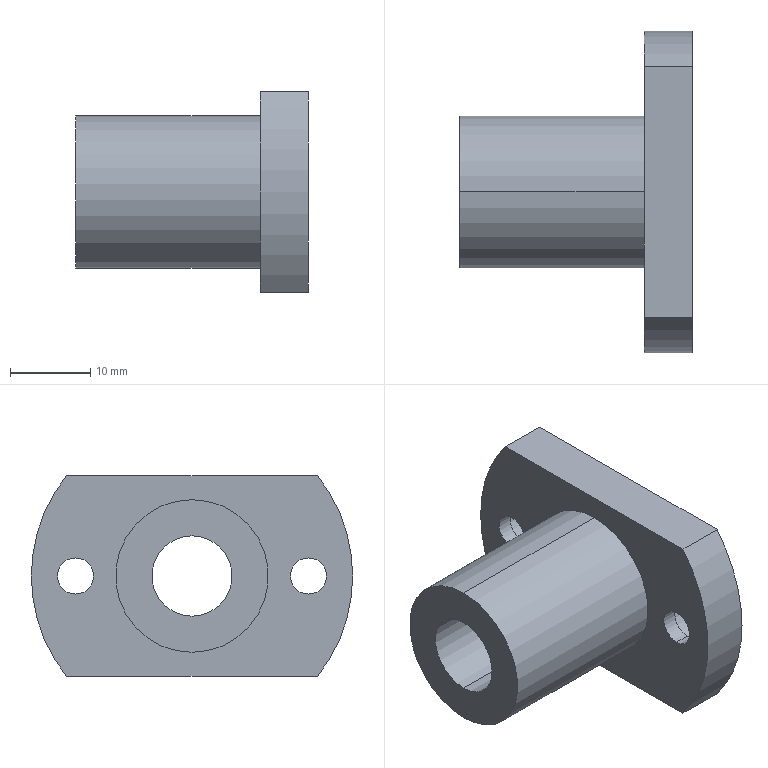Part | STEP file | Linear bearing LHFC 10 | 1 solid | 21 faces | box 29 x 40 x 25 mm | volume 9403 mm3 | cylinder 14 | plane 7 | commonest cylinder face diameters 4.5 x4 7.5 x4 10 x2 19 x2 40 x2
STEP:
#1=CARTESIAN_POINT('',(0.,0.,0.));
#2=DIRECTION('',(0.,0.,1.));
#3=DIRECTION('',(1.,0.,0.));
#4=AXIS2_PLACEMENT_3D('',#1,#2,#3);
#5=CARTESIAN_POINT('',(-23.,0.,9.5));
#6=VERTEX_POINT('',#5);
#7=CARTESIAN_POINT('',(-23.,0.,-9.5));
#8=VERTEX_POINT('',#7);
#9=CARTESIAN_POINT('',(-23.,0.,0.));
#10=DIRECTION('',(-1.,0.,0.));
#11=DIRECTION('',(0.,0.,-1.));
#12=AXIS2_PLACEMENT_3D('',#9,#10,#11);
#13=CIRCLE('',#12,9.5);
#14=CARTESIAN_POINT('',(-23.,0.,0.));
#15=DIRECTION('',(1.,0.,0.));
#16=DIRECTION('',(0.,0.,-1.));
#17=AXIS2_PLACEMENT_3D('',#14,#15,#16);
#18=CYLINDRICAL_SURFACE('',#17,9.5);
#19=CARTESIAN_POINT('',(6.283,0.));
#20=DIRECTION('',(-1.,0.));
#21=VECTOR('',#20,1.);
#22=LINE('',#19,#21);
#23=(GEOMETRIC_REPRESENTATION_CONTEXT(2)PARAMETRIC_REPRESENTATION_CONTEXT()REPRESENTATION_CONTEXT('',''));
#24=DEFINITIONAL_REPRESENTATION('',(#22),#23);
#25=PCURVE('',#18,#24);
#26=CARTESIAN_POINT('',(-23.,-9.614,-9.614));
#27=DIRECTION('',(-1.,0.,0.));
#28=DIRECTION('',(0.,0.,1.));
#29=AXIS2_PLACEMENT_3D('',#26,#27,#28);
#30=PLANE('',#29);
#31=CARTESIAN_POINT('',(9.614,9.614));
#32=DIRECTION('',(-1.,0.));
#33=AXIS2_PLACEMENT_2D('',#31,#32);
#34=CIRCLE('',#33,9.5);
#35=(GEOMETRIC_REPRESENTATION_CONTEXT(2)PARAMETRIC_REPRESENTATION_CONTEXT()REPRESENTATION_CONTEXT('',''));
#36=DEFINITIONAL_REPRESENTATION('',(#34),#35);
#37=PCURVE('',#30,#36);
#38=SURFACE_CURVE('',#13,(#25,#37),.PCURVE_S1.);
#39=EDGE_CURVE('',#6,#8,#38,.T.);
#40=ORIENTED_EDGE('',*,*,#39,.F.);
#41=CARTESIAN_POINT('',(0.,0.,9.5));
#42=VERTEX_POINT('',#41);
#43=CARTESIAN_POINT('',(-23.,0.,9.5));
#44=DIRECTION('',(1.,0.,0.));
#45=VECTOR('',#44,1.);
#46=LINE('',#43,#45);
#47=CARTESIAN_POINT('',(3.142,0.));
#48=DIRECTION('',(0.,1.));
#49=VECTOR('',#48,1.);
#50=LINE('',#47,#49);
#51=(GEOMETRIC_REPRESENTATION_CONTEXT(2)PARAMETRIC_REPRESENTATION_CONTEXT()REPRESENTATION_CONTEXT('',''));
#52=DEFINITIONAL_REPRESENTATION('',(#50),#51);
#53=PCURVE('',#18,#52);
#54=CARTESIAN_POINT('',(-23.,0.,0.));
#55=DIRECTION('',(1.,0.,0.));
#56=DIRECTION('',(0.,0.,-1.));
#57=AXIS2_PLACEMENT_3D('',#54,#55,#56);
#58=CYLINDRICAL_SURFACE('',#57,9.5);
#59=CARTESIAN_POINT('',(3.142,0.));
#60=DIRECTION('',(0.,1.));
#61=VECTOR('',#60,1.);
#62=LINE('',#59,#61);
#63=(GEOMETRIC_REPRESENTATION_CONTEXT(2)PARAMETRIC_REPRESENTATION_CONTEXT()REPRESENTATION_CONTEXT('',''));
#64=DEFINITIONAL_REPRESENTATION('',(#62),#63);
#65=PCURVE('',#58,#64);
#66=SURFACE_CURVE('',#46,(#53,#65),.PCURVE_S1.);
#67=EDGE_CURVE('',#6,#42,#66,.T.);
#68=ORIENTED_EDGE('',*,*,#67,.T.);
#69=CARTESIAN_POINT('',(0.,0.,-9.5));
#70=VERTEX_POINT('',#69);
#71=CARTESIAN_POINT('',(0.,0.,0.));
#72=DIRECTION('',(1.,0.,0.));
#73=DIRECTION('',(0.,0.,-1.));
#74=AXIS2_PLACEMENT_3D('',#71,#72,#73);
#75=CIRCLE('',#74,9.5);
#76=CARTESIAN_POINT('',(0.,23.));
#77=DIRECTION('',(1.,0.));
#78=VECTOR('',#77,1.);
#79=LINE('',#76,#78);
#80=(GEOMETRIC_REPRESENTATION_CONTEXT(2)PARAMETRIC_REPRESENTATION_CONTEXT()REPRESENTATION_CONTEXT('',''));
#81=DEFINITIONAL_REPRESENTATION('',(#79),#80);
#82=PCURVE('',#18,#81);
#83=CARTESIAN_POINT('',(0.,-20.24,12.5));
#84=DIRECTION('',(1.,0.,0.));
#85=DIRECTION('',(0.,0.,-1.));
#86=AXIS2_PLACEMENT_3D('',#83,#84,#85);
#87=PLANE('',#86);
#88=CARTESIAN_POINT('',(12.5,20.24));
#89=DIRECTION('',(1.,0.));
#90=AXIS2_PLACEMENT_2D('',#88,#89);
#91=CIRCLE('',#90,9.5);
#92=(GEOMETRIC_REPRESENTATION_CONTEXT(2)PARAMETRIC_REPRESENTATION_CONTEXT()REPRESENTATION_CONTEXT('',''));
#93=DEFINITIONAL_REPRESENTATION('',(#91),#92);
#94=PCURVE('',#87,#93);
#95=SURFACE_CURVE('',#75,(#82,#94),.PCURVE_S1.);
#96=EDGE_CURVE('',#70,#42,#95,.T.);
#97=ORIENTED_EDGE('',*,*,#96,.F.);
#98=CARTESIAN_POINT('',(-23.,0.,-9.5));
#99=DIRECTION('',(1.,0.,0.));
#100=VECTOR('',#99,1.);
#101=LINE('',#98,#100);
#102=CARTESIAN_POINT('',(0.,0.));
#103=DIRECTION('',(0.,1.));
#104=VECTOR('',#103,1.);
#105=LINE('',#102,#104);
#106=(GEOMETRIC_REPRESENTATION_CONTEXT(2)PARAMETRIC_REPRESENTATION_CONTEXT()REPRESENTATION_CONTEXT('',''));
#107=DEFINITIONAL_REPRESENTATION('',(#105),#106);
#108=PCURVE('',#18,#107);
#109=CARTESIAN_POINT('',(6.283,0.));
#110=DIRECTION('',(0.,1.));
#111=VECTOR('',#110,1.);
#112=LINE('',#109,#111);
#113=(GEOMETRIC_REPRESENTATION_CONTEXT(2)PARAMETRIC_REPRESENTATION_CONTEXT()REPRESENTATION_CONTEXT('',''));
#114=DEFINITIONAL_REPRESENTATION('',(#112),#113);
#115=PCURVE('',#58,#114);
#116=SURFACE_CURVE('',#101,(#108,#115),.PCURVE_S1.);
#117=EDGE_CURVE('',#8,#70,#116,.T.);
#118=ORIENTED_EDGE('',*,*,#117,.F.);
#119=EDGE_LOOP('',(#40,#68,#97,#118));
#120=FACE_BOUND('',#119,.T.);
#121=ADVANCED_FACE('',(#120),#18,.T.);
#122=CARTESIAN_POINT('',(6.,0.,5.));
#123=VERTEX_POINT('',#122);
#124=CARTESIAN_POINT('',(-23.,0.,5.));
#125=VERTEX_POINT('',#124);
#126=CARTESIAN_POINT('',(6.,0.,5.));
#127=DIRECTION('',(-1.,0.,0.));
#128=VECTOR('',#127,1.);
#129=LINE('',#126,#128);
#130=CARTESIAN_POINT('',(6.,0.,0.));
#131=DIRECTION('',(-1.,0.,0.));
#132=DIRECTION('',(0.,0.,1.));
#133=AXIS2_PLACEMENT_3D('',#130,#131,#132);
#134=CYLINDRICAL_SURFACE('',#133,5.);
#135=CARTESIAN_POINT('',(6.283,0.));
#136=DIRECTION('',(0.,1.));
#137=VECTOR('',#136,1.);
#138=LINE('',#135,#137);
#139=(GEOMETRIC_REPRESENTATION_CONTEXT(2)PARAMETRIC_REPRESENTATION_CONTEXT()REPRESENTATION_CONTEXT('',''));
#140=DEFINITIONAL_REPRESENTATION('',(#138),#139);
#141=PCURVE('',#134,#140);
#142=CARTESIAN_POINT('',(6.,0.,0.));
#143=DIRECTION('',(-1.,0.,0.));
#144=DIRECTION('',(0.,0.,1.));
#145=AXIS2_PLACEMENT_3D('',#142,#143,#144);
#146=CYLINDRICAL_SURFACE('',#145,5.);
#147=CARTESIAN_POINT('',(0.,0.));
#148=DIRECTION('',(0.,1.));
#149=VECTOR('',#148,1.);
#150=LINE('',#147,#149);
#151=(GEOMETRIC_REPRESENTATION_CONTEXT(2)PARAMETRIC_REPRESENTATION_CONTEXT()REPRESENTATION_CONTEXT('',''));
#152=DEFINITIONAL_REPRESENTATION('',(#150),#151);
#153=PCURVE('',#146,#152);
#154=SURFACE_CURVE('',#129,(#141,#153),.PCURVE_S1.);
#155=EDGE_CURVE('',#123,#125,#154,.T.);
#156=ORIENTED_EDGE('',*,*,#155,.T.);
#157=CARTESIAN_POINT('',(-23.,0.,-5.));
#158=VERTEX_POINT('',#157);
#159=CARTESIAN_POINT('',(-23.,0.,0.));
#160=DIRECTION('',(1.,0.,0.));
#161=DIRECTION('',(0.,0.,1.));
#162=AXIS2_PLACEMENT_3D('',#159,#160,#161);
#163=CIRCLE('',#162,5.);
#164=CARTESIAN_POINT('',(6.283,29.));
#165=DIRECTION('',(-1.,0.));
#166=VECTOR('',#165,1.);
#167=LINE('',#164,#166);
#168=(GEOMETRIC_REPRESENTATION_CONTEXT(2)PARAMETRIC_REPRESENTATION_CONTEXT()REPRESENTATION_CONTEXT('',''));
#169=DEFINITIONAL_REPRESENTATION('',(#167),#168);
#170=PCURVE('',#134,#169);
#171=CARTESIAN_POINT('',(14.614,9.614));
#172=CARTESIAN_POINT('',(14.614,0.9537));
#173=CARTESIAN_POINT('',(7.114,5.284));
#174=CARTESIAN_POINT('',(-0.386,9.614));
#175=CARTESIAN_POINT('',(7.114,13.944));
#176=CARTESIAN_POINT('',(14.614,18.274));
#177=CARTESIAN_POINT('',(14.614,9.614));
#178=(BOUNDED_CURVE()B_SPLINE_CURVE(2,(#171,#172,#173,#174,#175,#176,#177),.UNSPECIFIED.,.T.,.F.)B_SPLINE_CURVE_WITH_KNOTS((1,2,2,2,2,1),(-2.094,0.,2.094,4.189,6.283,8.378),.UNSPECIFIED.)CURVE()GEOMETRIC_REPRESENTATION_ITEM()RATIONAL_B_SPLINE_CURVE((1.,0.5,1.,0.5,1.,0.5,1.))REPRESENTATION_ITEM(''));
#179=(GEOMETRIC_REPRESENTATION_CONTEXT(2)PARAMETRIC_REPRESENTATION_CONTEXT()REPRESENTATION_CONTEXT('',''));
#180=DEFINITIONAL_REPRESENTATION('',(#178),#179);
#181=PCURVE('',#30,#180);
#182=SURFACE_CURVE('',#163,(#170,#181),.PCURVE_S1.);
#183=EDGE_CURVE('',#125,#158,#182,.T.);
#184=ORIENTED_EDGE('',*,*,#183,.T.);
#185=CARTESIAN_POINT('',(6.,0.,-5.));
#186=VERTEX_POINT('',#185);
#187=CARTESIAN_POINT('',(6.,0.,-5.));
#188=DIRECTION('',(-1.,0.,0.));
#189=VECTOR('',#188,1.);
#190=LINE('',#187,#189);
#191=CARTESIAN_POINT('',(3.142,0.));
#192=DIRECTION('',(0.,1.));
#193=VECTOR('',#192,1.);
#194=LINE('',#191,#193);
#195=(GEOMETRIC_REPRESENTATION_CONTEXT(2)PARAMETRIC_REPRESENTATION_CONTEXT()REPRESENTATION_CONTEXT('',''));
#196=DEFINITIONAL_REPRESENTATION('',(#194),#195);
#197=PCURVE('',#134,#196);
#198=CARTESIAN_POINT('',(3.142,0.));
#199=DIRECTION('',(0.,1.));
#200=VECTOR('',#199,1.);
#201=LINE('',#198,#200);
#202=(GEOMETRIC_REPRESENTATION_CONTEXT(2)PARAMETRIC_REPRESENTATION_CONTEXT()REPRESENTATION_CONTEXT('',''));
#203=DEFINITIONAL_REPRESENTATION('',(#201),#202);
#204=PCURVE('',#146,#203);
#205=SURFACE_CURVE('',#190,(#197,#204),.PCURVE_S1.);
#206=EDGE_CURVE('',#186,#158,#205,.T.);
#207=ORIENTED_EDGE('',*,*,#206,.F.);
#208=CARTESIAN_POINT('',(6.,0.,0.));
#209=DIRECTION('',(1.,0.,0.));
#210=DIRECTION('',(0.,0.,1.));
#211=AXIS2_PLACEMENT_3D('',#208,#209,#210);
#212=CIRCLE('',#211,5.);
#213=CARTESIAN_POINT('',(6.283,0.));
#214=DIRECTION('',(-1.,0.));
#215=VECTOR('',#214,1.);
#216=LINE('',#213,#215);
#217=(GEOMETRIC_REPRESENTATION_CONTEXT(2)PARAMETRIC_REPRESENTATION_CONTEXT()REPRESENTATION_CONTEXT('',''));
#218=DEFINITIONAL_REPRESENTATION('',(#216),#217);
#219=PCURVE('',#134,#218);
#220=CARTESIAN_POINT('',(6.,-20.24,12.5));
#221=DIRECTION('',(1.,0.,0.));
#222=DIRECTION('',(0.,0.,-1.));
#223=AXIS2_PLACEMENT_3D('',#220,#221,#222);
#224=PLANE('',#223);
#225=CARTESIAN_POINT('',(12.5,20.24));
#226=DIRECTION('',(-1.,0.));
#227=AXIS2_PLACEMENT_2D('',#225,#226);
#228=CIRCLE('',#227,5.);
#229=(GEOMETRIC_REPRESENTATION_CONTEXT(2)PARAMETRIC_REPRESENTATION_CONTEXT()REPRESENTATION_CONTEXT('',''));
#230=DEFINITIONAL_REPRESENTATION('',(#228),#229);
#231=PCURVE('',#224,#230);
#232=SURFACE_CURVE('',#212,(#219,#231),.PCURVE_S1.);
#233=EDGE_CURVE('',#123,#186,#232,.T.);
#234=ORIENTED_EDGE('',*,*,#233,.F.);
#235=EDGE_LOOP('',(#156,#184,#207,#234));
#236=FACE_BOUND('',#235,.F.);
#237=ADVANCED_FACE('',(#236),#134,.F.);
#238=CARTESIAN_POINT('',(0.,-14.5,-2.25));
#239=VERTEX_POINT('',#238);
#240=CARTESIAN_POINT('',(1.9,-14.5,-2.25));
#241=VERTEX_POINT('',#240);
#242=CARTESIAN_POINT('',(0.,-14.5,-2.25));
#243=DIRECTION('',(1.,0.,0.));
#244=VECTOR('',#243,1.);
#245=LINE('',#242,#244);
#246=CARTESIAN_POINT('',(0.,-14.5,0.));
#247=DIRECTION('',(1.,0.,0.));
#248=DIRECTION('',(0.,0.,-1.));
#249=AXIS2_PLACEMENT_3D('',#246,#247,#248);
#250=CYLINDRICAL_SURFACE('',#249,2.25);
#251=CARTESIAN_POINT('',(6.283,0.));
#252=DIRECTION('',(0.,1.));
#253=VECTOR('',#252,1.);
#254=LINE('',#251,#253);
#255=(GEOMETRIC_REPRESENTATION_CONTEXT(2)PARAMETRIC_REPRESENTATION_CONTEXT()REPRESENTATION_CONTEXT('',''));
#256=DEFINITIONAL_REPRESENTATION('',(#254),#255);
#257=PCURVE('',#250,#256);
#258=CARTESIAN_POINT('',(0.,-14.5,0.));
#259=DIRECTION('',(1.,0.,0.));
#260=DIRECTION('',(0.,0.,-1.));
#261=AXIS2_PLACEMENT_3D('',#258,#259,#260);
#262=CYLINDRICAL_SURFACE('',#261,2.25);
#263=CARTESIAN_POINT('',(0.,0.));
#264=DIRECTION('',(0.,1.));
#265=VECTOR('',#264,1.);
#266=LINE('',#263,#265);
#267=(GEOMETRIC_REPRESENTATION_CONTEXT(2)PARAMETRIC_REPRESENTATION_CONTEXT()REPRESENTATION_CONTEXT('',''));
#268=DEFINITIONAL_REPRESENTATION('',(#266),#267);
#269=PCURVE('',#262,#268);
#270=SURFACE_CURVE('',#245,(#257,#269),.PCURVE_S1.);
#271=EDGE_CURVE('',#239,#241,#270,.T.);
#272=ORIENTED_EDGE('',*,*,#271,.T.);
#273=CARTESIAN_POINT('',(1.9,-14.5,2.25));
#274=VERTEX_POINT('',#273);
#275=CARTESIAN_POINT('',(1.9,-14.5,0.));
#276=DIRECTION('',(1.,0.,0.));
#277=DIRECTION('',(0.,0.,-1.));
#278=AXIS2_PLACEMENT_3D('',#275,#276,#277);
#279=CIRCLE('',#278,2.25);
#280=CARTESIAN_POINT('',(0.,1.9));
#281=DIRECTION('',(1.,0.));
#282=VECTOR('',#281,1.);
#283=LINE('',#280,#282);
#284=(GEOMETRIC_REPRESENTATION_CONTEXT(2)PARAMETRIC_REPRESENTATION_CONTEXT()REPRESENTATION_CONTEXT('',''));
#285=DEFINITIONAL_REPRESENTATION('',(#283),#284);
#286=PCURVE('',#250,#285);
#287=CARTESIAN_POINT('',(1.9,-18.295,3.795));
#288=DIRECTION('',(1.,0.,0.));
#289=DIRECTION('',(0.,0.,-1.));
#290=AXIS2_PLACEMENT_3D('',#287,#288,#289);
#291=PLANE('',#290);
#292=CARTESIAN_POINT('',(3.795,3.795));
#293=DIRECTION('',(1.,0.));
#294=AXIS2_PLACEMENT_2D('',#292,#293);
#295=CIRCLE('',#294,2.25);
#296=(GEOMETRIC_REPRESENTATION_CONTEXT(2)PARAMETRIC_REPRESENTATION_CONTEXT()REPRESENTATION_CONTEXT('',''));
#297=DEFINITIONAL_REPRESENTATION('',(#295),#296);
#298=PCURVE('',#291,#297);
#299=SURFACE_CURVE('',#279,(#286,#298),.PCURVE_S1.);
#300=EDGE_CURVE('',#274,#241,#299,.T.);
#301=ORIENTED_EDGE('',*,*,#300,.F.);
#302=CARTESIAN_POINT('',(0.,-14.5,2.25));
#303=VERTEX_POINT('',#302);
#304=CARTESIAN_POINT('',(0.,-14.5,2.25));
#305=DIRECTION('',(1.,0.,0.));
#306=VECTOR('',#305,1.);
#307=LINE('',#304,#306);
#308=CARTESIAN_POINT('',(3.142,0.));
#309=DIRECTION('',(0.,1.));
#310=VECTOR('',#309,1.);
#311=LINE('',#308,#310);
#312=(GEOMETRIC_REPRESENTATION_CONTEXT(2)PARAMETRIC_REPRESENTATION_CONTEXT()REPRESENTATION_CONTEXT('',''));
#313=DEFINITIONAL_REPRESENTATION('',(#311),#312);
#314=PCURVE('',#250,#313);
#315=CARTESIAN_POINT('',(3.142,0.));
#316=DIRECTION('',(0.,1.));
#317=VECTOR('',#316,1.);
#318=LINE('',#315,#317);
#319=(GEOMETRIC_REPRESENTATION_CONTEXT(2)PARAMETRIC_REPRESENTATION_CONTEXT()REPRESENTATION_CONTEXT('',''));
#320=DEFINITIONAL_REPRESENTATION('',(#318),#319);
#321=PCURVE('',#262,#320);
#322=SURFACE_CURVE('',#307,(#314,#321),.PCURVE_S1.);
#323=EDGE_CURVE('',#303,#274,#322,.T.);
#324=ORIENTED_EDGE('',*,*,#323,.F.);
#325=CARTESIAN_POINT('',(0.,-14.5,0.));
#326=DIRECTION('',(-1.,0.,0.));
#327=DIRECTION('',(0.,0.,-1.));
#328=AXIS2_PLACEMENT_3D('',#325,#326,#327);
#329=CIRCLE('',#328,2.25);
#330=CARTESIAN_POINT('',(6.283,0.));
#331=DIRECTION('',(-1.,0.));
#332=VECTOR('',#331,1.);
#333=LINE('',#330,#332);
#334=(GEOMETRIC_REPRESENTATION_CONTEXT(2)PARAMETRIC_REPRESENTATION_CONTEXT()REPRESENTATION_CONTEXT('',''));
#335=DEFINITIONAL_REPRESENTATION('',(#333),#334);
#336=PCURVE('',#250,#335);
#337=CARTESIAN_POINT('',(14.75,5.74));
#338=CARTESIAN_POINT('',(14.75,1.843));
#339=CARTESIAN_POINT('',(11.375,3.791));
#340=CARTESIAN_POINT('',(8.,5.74));
#341=CARTESIAN_POINT('',(11.375,7.689));
#342=CARTESIAN_POINT('',(14.75,9.637));
#343=CARTESIAN_POINT('',(14.75,5.74));
#344=(BOUNDED_CURVE()B_SPLINE_CURVE(2,(#337,#338,#339,#340,#341,#342,#343),.UNSPECIFIED.,.T.,.F.)B_SPLINE_CURVE_WITH_KNOTS((1,2,2,2,2,1),(-2.094,0.,2.094,4.189,6.283,8.378),.UNSPECIFIED.)CURVE()GEOMETRIC_REPRESENTATION_ITEM()RATIONAL_B_SPLINE_CURVE((1.,0.5,1.,0.5,1.,0.5,1.))REPRESENTATION_ITEM(''));
#345=(GEOMETRIC_REPRESENTATION_CONTEXT(2)PARAMETRIC_REPRESENTATION_CONTEXT()REPRESENTATION_CONTEXT('',''));
#346=DEFINITIONAL_REPRESENTATION('',(#344),#345);
#347=PCURVE('',#87,#346);
#348=SURFACE_CURVE('',#329,(#336,#347),.PCURVE_S1.);
#349=EDGE_CURVE('',#239,#303,#348,.T.);
#350=ORIENTED_EDGE('',*,*,#349,.F.);
#351=EDGE_LOOP('',(#272,#301,#324,#350));
#352=FACE_BOUND('',#351,.F.);
#353=ADVANCED_FACE('',(#352),#250,.F.);
#354=CARTESIAN_POINT('',(0.,14.5,-2.25));
#355=VERTEX_POINT('',#354);
#356=CARTESIAN_POINT('',(1.9,14.5,-2.25));
#357=VERTEX_POINT('',#356);
#358=CARTESIAN_POINT('',(0.,14.5,-2.25));
#359=DIRECTION('',(1.,0.,0.));
#360=VECTOR('',#359,1.);
#361=LINE('',#358,#360);
#362=CARTESIAN_POINT('',(0.,14.5,0.));
#363=DIRECTION('',(1.,0.,0.));
#364=DIRECTION('',(0.,0.,-1.));
#365=AXIS2_PLACEMENT_3D('',#362,#363,#364);
#366=CYLINDRICAL_SURFACE('',#365,2.25);
#367=CARTESIAN_POINT('',(6.283,0.));
#368=DIRECTION('',(0.,1.));
#369=VECTOR('',#368,1.);
#370=LINE('',#367,#369);
#371=(GEOMETRIC_REPRESENTATION_CONTEXT(2)PARAMETRIC_REPRESENTATION_CONTEXT()REPRESENTATION_CONTEXT('',''));
#372=DEFINITIONAL_REPRESENTATION('',(#370),#371);
#373=PCURVE('',#366,#372);
#374=CARTESIAN_POINT('',(0.,14.5,0.));
#375=DIRECTION('',(1.,0.,0.));
#376=DIRECTION('',(0.,0.,-1.));
#377=AXIS2_PLACEMENT_3D('',#374,#375,#376);
#378=CYLINDRICAL_SURFACE('',#377,2.25);
#379=CARTESIAN_POINT('',(0.,0.));
#380=DIRECTION('',(0.,1.));
#381=VECTOR('',#380,1.);
#382=LINE('',#379,#381);
#383=(GEOMETRIC_REPRESENTATION_CONTEXT(2)PARAMETRIC_REPRESENTATION_CONTEXT()REPRESENTATION_CONTEXT('',''));
#384=DEFINITIONAL_REPRESENTATION('',(#382),#383);
#385=PCURVE('',#378,#384);
#386=SURFACE_CURVE('',#361,(#373,#385),.PCURVE_S1.);
#387=EDGE_CURVE('',#355,#357,#386,.T.);
#388=ORIENTED_EDGE('',*,*,#387,.T.);
#389=CARTESIAN_POINT('',(1.9,14.5,2.25));
#390=VERTEX_POINT('',#389);
#391=CARTESIAN_POINT('',(1.9,14.5,0.));
#392=DIRECTION('',(1.,0.,0.));
#393=DIRECTION('',(0.,0.,-1.));
#394=AXIS2_PLACEMENT_3D('',#391,#392,#393);
#395=CIRCLE('',#394,2.25);
#396=CARTESIAN_POINT('',(0.,1.9));
#397=DIRECTION('',(1.,0.));
#398=VECTOR('',#397,1.);
#399=LINE('',#396,#398);
#400=(GEOMETRIC_REPRESENTATION_CONTEXT(2)PARAMETRIC_REPRESENTATION_CONTEXT()REPRESENTATION_CONTEXT('',''));
#401=DEFINITIONAL_REPRESENTATION('',(#399),#400);
#402=PCURVE('',#366,#401);
#403=CARTESIAN_POINT('',(1.9,10.705,3.795));
#404=DIRECTION('',(1.,0.,0.));
#405=DIRECTION('',(0.,0.,-1.));
#406=AXIS2_PLACEMENT_3D('',#403,#404,#405);
#407=PLANE('',#406);
#408=CARTESIAN_POINT('',(3.795,3.795));
#409=DIRECTION('',(1.,0.));
#410=AXIS2_PLACEMENT_2D('',#408,#409);
#411=CIRCLE('',#410,2.25);
#412=(GEOMETRIC_REPRESENTATION_CONTEXT(2)PARAMETRIC_REPRESENTATION_CONTEXT()REPRESENTATION_CONTEXT('',''));
#413=DEFINITIONAL_REPRESENTATION('',(#411),#412);
#414=PCURVE('',#407,#413);
#415=SURFACE_CURVE('',#395,(#402,#414),.PCURVE_S1.);
#416=EDGE_CURVE('',#390,#357,#415,.T.);
#417=ORIENTED_EDGE('',*,*,#416,.F.);
#418=CARTESIAN_POINT('',(0.,14.5,2.25));
#419=VERTEX_POINT('',#418);
#420=CARTESIAN_POINT('',(0.,14.5,2.25));
#421=DIRECTION('',(1.,0.,0.));
#422=VECTOR('',#421,1.);
#423=LINE('',#420,#422);
#424=CARTESIAN_POINT('',(3.142,0.));
#425=DIRECTION('',(0.,1.));
#426=VECTOR('',#425,1.);
#427=LINE('',#424,#426);
#428=(GEOMETRIC_REPRESENTATION_CONTEXT(2)PARAMETRIC_REPRESENTATION_CONTEXT()REPRESENTATION_CONTEXT('',''));
#429=DEFINITIONAL_REPRESENTATION('',(#427),#428);
#430=PCURVE('',#366,#429);
#431=CARTESIAN_POINT('',(3.142,0.));
#432=DIRECTION('',(0.,1.));
#433=VECTOR('',#432,1.);
#434=LINE('',#431,#433);
#435=(GEOMETRIC_REPRESENTATION_CONTEXT(2)PARAMETRIC_REPRESENTATION_CONTEXT()REPRESENTATION_CONTEXT('',''));
#436=DEFINITIONAL_REPRESENTATION('',(#434),#435);
#437=PCURVE('',#378,#436);
#438=SURFACE_CURVE('',#423,(#430,#437),.PCURVE_S1.);
#439=EDGE_CURVE('',#419,#390,#438,.T.);
#440=ORIENTED_EDGE('',*,*,#439,.F.);
#441=CARTESIAN_POINT('',(0.,14.5,0.));
#442=DIRECTION('',(-1.,0.,0.));
#443=DIRECTION('',(0.,0.,-1.));
#444=AXIS2_PLACEMENT_3D('',#441,#442,#443);
#445=CIRCLE('',#444,2.25);
#446=CARTESIAN_POINT('',(6.283,0.));
#447=DIRECTION('',(-1.,0.));
#448=VECTOR('',#447,1.);
#449=LINE('',#446,#448);
#450=(GEOMETRIC_REPRESENTATION_CONTEXT(2)PARAMETRIC_REPRESENTATION_CONTEXT()REPRESENTATION_CONTEXT('',''));
#451=DEFINITIONAL_REPRESENTATION('',(#449),#450);
#452=PCURVE('',#366,#451);
#453=CARTESIAN_POINT('',(14.75,34.74));
#454=CARTESIAN_POINT('',(14.75,30.843));
#455=CARTESIAN_POINT('',(11.375,32.791));
#456=CARTESIAN_POINT('',(8.,34.74));
#457=CARTESIAN_POINT('',(11.375,36.689));
#458=CARTESIAN_POINT('',(14.75,38.637));
#459=CARTESIAN_POINT('',(14.75,34.74));
#460=(BOUNDED_CURVE()B_SPLINE_CURVE(2,(#453,#454,#455,#456,#457,#458,#459),.UNSPECIFIED.,.T.,.F.)B_SPLINE_CURVE_WITH_KNOTS((1,2,2,2,2,1),(-2.094,0.,2.094,4.189,6.283,8.378),.UNSPECIFIED.)CURVE()GEOMETRIC_REPRESENTATION_ITEM()RATIONAL_B_SPLINE_CURVE((1.,0.5,1.,0.5,1.,0.5,1.))REPRESENTATION_ITEM(''));
#461=(GEOMETRIC_REPRESENTATION_CONTEXT(2)PARAMETRIC_REPRESENTATION_CONTEXT()REPRESENTATION_CONTEXT('',''));
#462=DEFINITIONAL_REPRESENTATION('',(#460),#461);
#463=PCURVE('',#87,#462);
#464=SURFACE_CURVE('',#445,(#452,#463),.PCURVE_S1.);
#465=EDGE_CURVE('',#355,#419,#464,.T.);
#466=ORIENTED_EDGE('',*,*,#465,.F.);
#467=EDGE_LOOP('',(#388,#417,#440,#466));
#468=FACE_BOUND('',#467,.F.);
#469=ADVANCED_FACE('',(#468),#366,.F.);
#470=CARTESIAN_POINT('',(1.9,18.25,0.));
#471=VERTEX_POINT('',#470);
#472=CARTESIAN_POINT('',(6.,18.25,0.));
#473=VERTEX_POINT('',#472);
#474=CARTESIAN_POINT('',(1.9,18.25,0.));
#475=DIRECTION('',(1.,0.,0.));
#476=VECTOR('',#475,1.);
#477=LINE('',#474,#476);
#478=CARTESIAN_POINT('',(1.9,14.5,0.));
#479=DIRECTION('',(1.,0.,0.));
#480=DIRECTION('',(0.,1.,0.));
#481=AXIS2_PLACEMENT_3D('',#478,#479,#480);
#482=CYLINDRICAL_SURFACE('',#481,3.75);
#483=CARTESIAN_POINT('',(6.283,0.));
#484=DIRECTION('',(0.,1.));
#485=VECTOR('',#484,1.);
#486=LINE('',#483,#485);
#487=(GEOMETRIC_REPRESENTATION_CONTEXT(2)PARAMETRIC_REPRESENTATION_CONTEXT()REPRESENTATION_CONTEXT('',''));
#488=DEFINITIONAL_REPRESENTATION('',(#486),#487);
#489=PCURVE('',#482,#488);
#490=CARTESIAN_POINT('',(1.9,14.5,0.));
#491=DIRECTION('',(1.,0.,0.));
#492=DIRECTION('',(0.,1.,0.));
#493=AXIS2_PLACEMENT_3D('',#490,#491,#492);
#494=CYLINDRICAL_SURFACE('',#493,3.75);
#495=CARTESIAN_POINT('',(0.,0.));
#496=DIRECTION('',(0.,1.));
#497=VECTOR('',#496,1.);
#498=LINE('',#495,#497);
#499=(GEOMETRIC_REPRESENTATION_CONTEXT(2)PARAMETRIC_REPRESENTATION_CONTEXT()REPRESENTATION_CONTEXT('',''));
#500=DEFINITIONAL_REPRESENTATION('',(#498),#499);
#501=PCURVE('',#494,#500);
#502=SURFACE_CURVE('',#477,(#489,#501),.PCURVE_S1.);
#503=EDGE_CURVE('',#471,#473,#502,.T.);
#504=ORIENTED_EDGE('',*,*,#503,.T.);
#505=CARTESIAN_POINT('',(6.,10.75,0.));
#506=VERTEX_POINT('',#505);
#507=CARTESIAN_POINT('',(6.,14.5,0.));
#508=DIRECTION('',(-1.,0.,0.));
#509=DIRECTION('',(0.,1.,0.));
#510=AXIS2_PLACEMENT_3D('',#507,#508,#509);
#511=CIRCLE('',#510,3.75);
#512=CARTESIAN_POINT('',(6.283,4.1));
#513=DIRECTION('',(-1.,0.));
#514=VECTOR('',#513,1.);
#515=LINE('',#512,#514);
#516=(GEOMETRIC_REPRESENTATION_CONTEXT(2)PARAMETRIC_REPRESENTATION_CONTEXT()REPRESENTATION_CONTEXT('',''));
#517=DEFINITIONAL_REPRESENTATION('',(#515),#516);
#518=PCURVE('',#482,#517);
#519=CARTESIAN_POINT('',(12.5,38.49));
#520=CARTESIAN_POINT('',(18.995,38.49));
#521=CARTESIAN_POINT('',(15.748,32.865));
#522=CARTESIAN_POINT('',(12.5,27.24));
#523=CARTESIAN_POINT('',(9.252,32.865));
#524=CARTESIAN_POINT('',(6.005,38.49));
#525=CARTESIAN_POINT('',(12.5,38.49));
#526=(BOUNDED_CURVE()B_SPLINE_CURVE(2,(#519,#520,#521,#522,#523,#524,#525),.UNSPECIFIED.,.T.,.F.)B_SPLINE_CURVE_WITH_KNOTS((1,2,2,2,2,1),(-2.094,0.,2.094,4.189,6.283,8.378),.UNSPECIFIED.)CURVE()GEOMETRIC_REPRESENTATION_ITEM()RATIONAL_B_SPLINE_CURVE((1.,0.5,1.,0.5,1.,0.5,1.))REPRESENTATION_ITEM(''));
#527=(GEOMETRIC_REPRESENTATION_CONTEXT(2)PARAMETRIC_REPRESENTATION_CONTEXT()REPRESENTATION_CONTEXT('',''));
#528=DEFINITIONAL_REPRESENTATION('',(#526),#527);
#529=PCURVE('',#224,#528);
#530=SURFACE_CURVE('',#511,(#518,#529),.PCURVE_S1.);
#531=EDGE_CURVE('',#473,#506,#530,.T.);
#532=ORIENTED_EDGE('',*,*,#531,.T.);
#533=CARTESIAN_POINT('',(1.9,10.75,0.));
#534=VERTEX_POINT('',#533);
#535=CARTESIAN_POINT('',(1.9,10.75,0.));
#536=DIRECTION('',(1.,0.,0.));
#537=VECTOR('',#536,1.);
#538=LINE('',#535,#537);
#539=CARTESIAN_POINT('',(3.142,0.));
#540=DIRECTION('',(0.,1.));
#541=VECTOR('',#540,1.);
#542=LINE('',#539,#541);
#543=(GEOMETRIC_REPRESENTATION_CONTEXT(2)PARAMETRIC_REPRESENTATION_CONTEXT()REPRESENTATION_CONTEXT('',''));
#544=DEFINITIONAL_REPRESENTATION('',(#542),#543);
#545=PCURVE('',#482,#544);
#546=CARTESIAN_POINT('',(3.142,0.));
#547=DIRECTION('',(0.,1.));
#548=VECTOR('',#547,1.);
#549=LINE('',#546,#548);
#550=(GEOMETRIC_REPRESENTATION_CONTEXT(2)PARAMETRIC_REPRESENTATION_CONTEXT()REPRESENTATION_CONTEXT('',''));
#551=DEFINITIONAL_REPRESENTATION('',(#549),#550);
#552=PCURVE('',#494,#551);
#553=SURFACE_CURVE('',#538,(#545,#552),.PCURVE_S1.);
#554=EDGE_CURVE('',#534,#506,#553,.T.);
#555=ORIENTED_EDGE('',*,*,#554,.F.);
#556=CARTESIAN_POINT('',(1.9,14.5,0.));
#557=DIRECTION('',(1.,0.,0.));
#558=DIRECTION('',(0.,1.,0.));
#559=AXIS2_PLACEMENT_3D('',#556,#557,#558);
#560=CIRCLE('',#559,3.75);
#561=CARTESIAN_POINT('',(0.,0.));
#562=DIRECTION('',(1.,0.));
#563=VECTOR('',#562,1.);
#564=LINE('',#561,#563);
#565=(GEOMETRIC_REPRESENTATION_CONTEXT(2)PARAMETRIC_REPRESENTATION_CONTEXT()REPRESENTATION_CONTEXT('',''));
#566=DEFINITIONAL_REPRESENTATION('',(#564),#565);
#567=PCURVE('',#482,#566);
#568=CARTESIAN_POINT('',(3.795,3.795));
#569=DIRECTION('',(0.,1.));
#570=AXIS2_PLACEMENT_2D('',#568,#569);
#571=CIRCLE('',#570,3.75);
#572=(GEOMETRIC_REPRESENTATION_CONTEXT(2)PARAMETRIC_REPRESENTATION_CONTEXT()REPRESENTATION_CONTEXT('',''));
#573=DEFINITIONAL_REPRESENTATION('',(#571),#572);
#574=PCURVE('',#407,#573);
#575=SURFACE_CURVE('',#560,(#567,#574),.PCURVE_S1.);
#576=EDGE_CURVE('',#534,#471,#575,.T.);
#577=ORIENTED_EDGE('',*,*,#576,.T.);
#578=EDGE_LOOP('',(#504,#532,#555,#577));
#579=FACE_BOUND('',#578,.F.);
#580=ADVANCED_FACE('',(#579),#482,.F.);
#581=CARTESIAN_POINT('',(1.9,-10.75,0.));
#582=VERTEX_POINT('',#581);
#583=CARTESIAN_POINT('',(6.,-10.75,0.));
#584=VERTEX_POINT('',#583);
#585=CARTESIAN_POINT('',(1.9,-10.75,0.));
#586=DIRECTION('',(1.,0.,0.));
#587=VECTOR('',#586,1.);
#588=LINE('',#585,#587);
#589=CARTESIAN_POINT('',(1.9,-14.5,0.));
#590=DIRECTION('',(1.,0.,0.));
#591=DIRECTION('',(0.,1.,0.));
#592=AXIS2_PLACEMENT_3D('',#589,#590,#591);
#593=CYLINDRICAL_SURFACE('',#592,3.75);
#594=CARTESIAN_POINT('',(6.283,0.));
#595=DIRECTION('',(0.,1.));
#596=VECTOR('',#595,1.);
#597=LINE('',#594,#596);
#598=(GEOMETRIC_REPRESENTATION_CONTEXT(2)PARAMETRIC_REPRESENTATION_CONTEXT()REPRESENTATION_CONTEXT('',''));
#599=DEFINITIONAL_REPRESENTATION('',(#597),#598);
#600=PCURVE('',#593,#599);
#601=CARTESIAN_POINT('',(1.9,-14.5,0.));
#602=DIRECTION('',(1.,0.,0.));
#603=DIRECTION('',(0.,1.,0.));
#604=AXIS2_PLACEMENT_3D('',#601,#602,#603);
#605=CYLINDRICAL_SURFACE('',#604,3.75);
#606=CARTESIAN_POINT('',(0.,0.));
#607=DIRECTION('',(0.,1.));
#608=VECTOR('',#607,1.);
#609=LINE('',#606,#608);
#610=(GEOMETRIC_REPRESENTATION_CONTEXT(2)PARAMETRIC_REPRESENTATION_CONTEXT()REPRESENTATION_CONTEXT('',''));
#611=DEFINITIONAL_REPRESENTATION('',(#609),#610);
#612=PCURVE('',#605,#611);
#613=SURFACE_CURVE('',#588,(#600,#612),.PCURVE_S1.);
#614=EDGE_CURVE('',#582,#584,#613,.T.);
#615=ORIENTED_EDGE('',*,*,#614,.T.);
#616=CARTESIAN_POINT('',(6.,-18.25,0.));
#617=VERTEX_POINT('',#616);
#618=CARTESIAN_POINT('',(6.,-14.5,0.));
#619=DIRECTION('',(-1.,0.,0.));
#620=DIRECTION('',(0.,1.,0.));
#621=AXIS2_PLACEMENT_3D('',#618,#619,#620);
#622=CIRCLE('',#621,3.75);
#623=CARTESIAN_POINT('',(6.283,4.1));
#624=DIRECTION('',(-1.,0.));
#625=VECTOR('',#624,1.);
#626=LINE('',#623,#625);
#627=(GEOMETRIC_REPRESENTATION_CONTEXT(2)PARAMETRIC_REPRESENTATION_CONTEXT()REPRESENTATION_CONTEXT('',''));
#628=DEFINITIONAL_REPRESENTATION('',(#626),#627);
#629=PCURVE('',#593,#628);
#630=CARTESIAN_POINT('',(12.5,9.49));
#631=CARTESIAN_POINT('',(18.995,9.49));
#632=CARTESIAN_POINT('',(15.748,3.865));
#633=CARTESIAN_POINT('',(12.5,-1.76));
#634=CARTESIAN_POINT('',(9.252,3.865));
#635=CARTESIAN_POINT('',(6.005,9.49));
#636=CARTESIAN_POINT('',(12.5,9.49));
#637=(BOUNDED_CURVE()B_SPLINE_CURVE(2,(#630,#631,#632,#633,#634,#635,#636),.UNSPECIFIED.,.T.,.F.)B_SPLINE_CURVE_WITH_KNOTS((1,2,2,2,2,1),(-2.094,0.,2.094,4.189,6.283,8.378),.UNSPECIFIED.)CURVE()GEOMETRIC_REPRESENTATION_ITEM()RATIONAL_B_SPLINE_CURVE((1.,0.5,1.,0.5,1.,0.5,1.))REPRESENTATION_ITEM(''));
#638=(GEOMETRIC_REPRESENTATION_CONTEXT(2)PARAMETRIC_REPRESENTATION_CONTEXT()REPRESENTATION_CONTEXT('',''));
#639=DEFINITIONAL_REPRESENTATION('',(#637),#638);
#640=PCURVE('',#224,#639);
#641=SURFACE_CURVE('',#622,(#629,#640),.PCURVE_S1.);
#642=EDGE_CURVE('',#584,#617,#641,.T.);
#643=ORIENTED_EDGE('',*,*,#642,.T.);
#644=CARTESIAN_POINT('',(1.9,-18.25,0.));
#645=VERTEX_POINT('',#644);
#646=CARTESIAN_POINT('',(1.9,-18.25,0.));
#647=DIRECTION('',(1.,0.,0.));
#648=VECTOR('',#647,1.);
#649=LINE('',#646,#648);
#650=CARTESIAN_POINT('',(3.142,0.));
#651=DIRECTION('',(0.,1.));
#652=VECTOR('',#651,1.);
#653=LINE('',#650,#652);
#654=(GEOMETRIC_REPRESENTATION_CONTEXT(2)PARAMETRIC_REPRESENTATION_CONTEXT()REPRESENTATION_CONTEXT('',''));
#655=DEFINITIONAL_REPRESENTATION('',(#653),#654);
#656=PCURVE('',#593,#655);
#657=CARTESIAN_POINT('',(3.142,0.));
#658=DIRECTION('',(0.,1.));
#659=VECTOR('',#658,1.);
#660=LINE('',#657,#659);
#661=(GEOMETRIC_REPRESENTATION_CONTEXT(2)PARAMETRIC_REPRESENTATION_CONTEXT()REPRESENTATION_CONTEXT('',''));
#662=DEFINITIONAL_REPRESENTATION('',(#660),#661);
#663=PCURVE('',#605,#662);
#664=SURFACE_CURVE('',#649,(#656,#663),.PCURVE_S1.);
#665=EDGE_CURVE('',#645,#617,#664,.T.);
#666=ORIENTED_EDGE('',*,*,#665,.F.);
#667=CARTESIAN_POINT('',(1.9,-14.5,0.));
#668=DIRECTION('',(1.,0.,0.));
#669=DIRECTION('',(0.,1.,0.));
#670=AXIS2_PLACEMENT_3D('',#667,#668,#669);
#671=CIRCLE('',#670,3.75);
#672=CARTESIAN_POINT('',(0.,0.));
#673=DIRECTION('',(1.,0.));
#674=VECTOR('',#673,1.);
#675=LINE('',#672,#674);
#676=(GEOMETRIC_REPRESENTATION_CONTEXT(2)PARAMETRIC_REPRESENTATION_CONTEXT()REPRESENTATION_CONTEXT('',''));
#677=DEFINITIONAL_REPRESENTATION('',(#675),#676);
#678=PCURVE('',#593,#677);
#679=CARTESIAN_POINT('',(3.795,3.795));
#680=DIRECTION('',(0.,1.));
#681=AXIS2_PLACEMENT_2D('',#679,#680);
#682=CIRCLE('',#681,3.75);
#683=(GEOMETRIC_REPRESENTATION_CONTEXT(2)PARAMETRIC_REPRESENTATION_CONTEXT()REPRESENTATION_CONTEXT('',''));
#684=DEFINITIONAL_REPRESENTATION('',(#682),#683);
#685=PCURVE('',#291,#684);
#686=SURFACE_CURVE('',#671,(#678,#685),.PCURVE_S1.);
#687=EDGE_CURVE('',#645,#582,#686,.T.);
#688=ORIENTED_EDGE('',*,*,#687,.T.);
#689=EDGE_LOOP('',(#615,#643,#666,#688));
#690=FACE_BOUND('',#689,.F.);
#691=ADVANCED_FACE('',(#690),#593,.F.);
#692=ORIENTED_EDGE('',*,*,#67,.F.);
#693=CARTESIAN_POINT('',(-23.,0.,0.));
#694=DIRECTION('',(-1.,0.,0.));
#695=DIRECTION('',(0.,0.,-1.));
#696=AXIS2_PLACEMENT_3D('',#693,#694,#695);
#697=CIRCLE('',#696,9.5);
#698=CARTESIAN_POINT('',(6.283,0.));
#699=DIRECTION('',(-1.,0.));
#700=VECTOR('',#699,1.);
#701=LINE('',#698,#700);
#702=(GEOMETRIC_REPRESENTATION_CONTEXT(2)PARAMETRIC_REPRESENTATION_CONTEXT()REPRESENTATION_CONTEXT('',''));
#703=DEFINITIONAL_REPRESENTATION('',(#701),#702);
#704=PCURVE('',#58,#703);
#705=CARTESIAN_POINT('',(9.614,9.614));
#706=DIRECTION('',(-1.,0.));
#707=AXIS2_PLACEMENT_2D('',#705,#706);
#708=CIRCLE('',#707,9.5);
#709=(GEOMETRIC_REPRESENTATION_CONTEXT(2)PARAMETRIC_REPRESENTATION_CONTEXT()REPRESENTATION_CONTEXT('',''));
#710=DEFINITIONAL_REPRESENTATION('',(#708),#709);
#711=PCURVE('',#30,#710);
#712=SURFACE_CURVE('',#697,(#704,#711),.PCURVE_S1.);
#713=EDGE_CURVE('',#8,#6,#712,.T.);
#714=ORIENTED_EDGE('',*,*,#713,.F.);
#715=ORIENTED_EDGE('',*,*,#117,.T.);
#716=CARTESIAN_POINT('',(0.,0.,0.));
#717=DIRECTION('',(1.,0.,0.));
#718=DIRECTION('',(0.,0.,-1.));
#719=AXIS2_PLACEMENT_3D('',#716,#717,#718);
#720=CIRCLE('',#719,9.5);
#721=CARTESIAN_POINT('',(0.,23.));
#722=DIRECTION('',(1.,0.));
#723=VECTOR('',#722,1.);
#724=LINE('',#721,#723);
#725=(GEOMETRIC_REPRESENTATION_CONTEXT(2)PARAMETRIC_REPRESENTATION_CONTEXT()REPRESENTATION_CONTEXT('',''));
#726=DEFINITIONAL_REPRESENTATION('',(#724),#725);
#727=PCURVE('',#58,#726);
#728=CARTESIAN_POINT('',(12.5,20.24));
#729=DIRECTION('',(1.,0.));
#730=AXIS2_PLACEMENT_2D('',#728,#729);
#731=CIRCLE('',#730,9.5);
#732=(GEOMETRIC_REPRESENTATION_CONTEXT(2)PARAMETRIC_REPRESENTATION_CONTEXT()REPRESENTATION_CONTEXT('',''));
#733=DEFINITIONAL_REPRESENTATION('',(#731),#732);
#734=PCURVE('',#87,#733);
#735=SURFACE_CURVE('',#720,(#727,#734),.PCURVE_S1.);
#736=EDGE_CURVE('',#42,#70,#735,.T.);
#737=ORIENTED_EDGE('',*,*,#736,.F.);
#738=EDGE_LOOP('',(#692,#714,#715,#737));
#739=FACE_BOUND('',#738,.T.);
#740=ADVANCED_FACE('',(#739),#58,.T.);
#741=ORIENTED_EDGE('',*,*,#183,.T.);
#742=CARTESIAN_POINT('',(-23.,0.,0.));
#743=DIRECTION('',(1.,0.,0.));
#744=DIRECTION('',(0.,0.,1.));
#745=AXIS2_PLACEMENT_3D('',#742,#743,#744);
#746=CIRCLE('',#745,5.);
#747=CARTESIAN_POINT('',(14.614,9.614));
#748=CARTESIAN_POINT('',(14.614,0.9537));
#749=CARTESIAN_POINT('',(7.114,5.284));
#750=CARTESIAN_POINT('',(-0.386,9.614));
#751=CARTESIAN_POINT('',(7.114,13.944));
#752=CARTESIAN_POINT('',(14.614,18.274));
#753=CARTESIAN_POINT('',(14.614,9.614));
#754=(BOUNDED_CURVE()B_SPLINE_CURVE(2,(#747,#748,#749,#750,#751,#752,#753),.UNSPECIFIED.,.T.,.F.)B_SPLINE_CURVE_WITH_KNOTS((1,2,2,2,2,1),(-2.094,0.,2.094,4.189,6.283,8.378),.UNSPECIFIED.)CURVE()GEOMETRIC_REPRESENTATION_ITEM()RATIONAL_B_SPLINE_CURVE((1.,0.5,1.,0.5,1.,0.5,1.))REPRESENTATION_ITEM(''));
#755=(GEOMETRIC_REPRESENTATION_CONTEXT(2)PARAMETRIC_REPRESENTATION_CONTEXT()REPRESENTATION_CONTEXT('',''));
#756=DEFINITIONAL_REPRESENTATION('',(#754),#755);
#757=PCURVE('',#30,#756);
#758=CARTESIAN_POINT('',(6.283,29.));
#759=DIRECTION('',(-1.,0.));
#760=VECTOR('',#759,1.);
#761=LINE('',#758,#760);
#762=(GEOMETRIC_REPRESENTATION_CONTEXT(2)PARAMETRIC_REPRESENTATION_CONTEXT()REPRESENTATION_CONTEXT('',''));
#763=DEFINITIONAL_REPRESENTATION('',(#761),#762);
#764=PCURVE('',#146,#763);
#765=SURFACE_CURVE('',#746,(#757,#764),.PCURVE_S1.);
#766=EDGE_CURVE('',#158,#125,#765,.T.);
#767=ORIENTED_EDGE('',*,*,#766,.T.);
#768=EDGE_LOOP('',(#741,#767));
#769=FACE_BOUND('',#768,.T.);
#770=ORIENTED_EDGE('',*,*,#713,.T.);
#771=ORIENTED_EDGE('',*,*,#39,.T.);
#772=EDGE_LOOP('',(#770,#771));
#773=FACE_BOUND('',#772,.T.);
#774=ADVANCED_FACE('',(#769,#773),#30,.T.);
#775=ORIENTED_EDGE('',*,*,#96,.T.);
#776=ORIENTED_EDGE('',*,*,#736,.T.);
#777=EDGE_LOOP('',(#775,#776));
#778=FACE_BOUND('',#777,.T.);
#779=ORIENTED_EDGE('',*,*,#349,.F.);
#780=CARTESIAN_POINT('',(0.,-14.5,0.));
#781=DIRECTION('',(-1.,0.,0.));
#782=DIRECTION('',(0.,0.,-1.));
#783=AXIS2_PLACEMENT_3D('',#780,#781,#782);
#784=CIRCLE('',#783,2.25);
#785=CARTESIAN_POINT('',(14.75,5.74));
#786=CARTESIAN_POINT('',(14.75,1.843));
#787=CARTESIAN_POINT('',(11.375,3.791));
#788=CARTESIAN_POINT('',(8.,5.74));
#789=CARTESIAN_POINT('',(11.375,7.689));
#790=CARTESIAN_POINT('',(14.75,9.637));
#791=CARTESIAN_POINT('',(14.75,5.74));
#792=(BOUNDED_CURVE()B_SPLINE_CURVE(2,(#785,#786,#787,#788,#789,#790,#791),.UNSPECIFIED.,.T.,.F.)B_SPLINE_CURVE_WITH_KNOTS((1,2,2,2,2,1),(-2.094,0.,2.094,4.189,6.283,8.378),.UNSPECIFIED.)CURVE()GEOMETRIC_REPRESENTATION_ITEM()RATIONAL_B_SPLINE_CURVE((1.,0.5,1.,0.5,1.,0.5,1.))REPRESENTATION_ITEM(''));
#793=(GEOMETRIC_REPRESENTATION_CONTEXT(2)PARAMETRIC_REPRESENTATION_CONTEXT()REPRESENTATION_CONTEXT('',''));
#794=DEFINITIONAL_REPRESENTATION('',(#792),#793);
#795=PCURVE('',#87,#794);
#796=CARTESIAN_POINT('',(6.283,0.));
#797=DIRECTION('',(-1.,0.));
#798=VECTOR('',#797,1.);
#799=LINE('',#796,#798);
#800=(GEOMETRIC_REPRESENTATION_CONTEXT(2)PARAMETRIC_REPRESENTATION_CONTEXT()REPRESENTATION_CONTEXT('',''));
#801=DEFINITIONAL_REPRESENTATION('',(#799),#800);
#802=PCURVE('',#262,#801);
#803=SURFACE_CURVE('',#784,(#795,#802),.PCURVE_S1.);
#804=EDGE_CURVE('',#303,#239,#803,.T.);
#805=ORIENTED_EDGE('',*,*,#804,.F.);
#806=EDGE_LOOP('',(#779,#805));
#807=FACE_BOUND('',#806,.T.);
#808=ORIENTED_EDGE('',*,*,#465,.F.);
#809=CARTESIAN_POINT('',(0.,14.5,0.));
#810=DIRECTION('',(-1.,0.,0.));
#811=DIRECTION('',(0.,0.,-1.));
#812=AXIS2_PLACEMENT_3D('',#809,#810,#811);
#813=CIRCLE('',#812,2.25);
#814=CARTESIAN_POINT('',(14.75,34.74));
#815=CARTESIAN_POINT('',(14.75,30.843));
#816=CARTESIAN_POINT('',(11.375,32.791));
#817=CARTESIAN_POINT('',(8.,34.74));
#818=CARTESIAN_POINT('',(11.375,36.689));
#819=CARTESIAN_POINT('',(14.75,38.637));
#820=CARTESIAN_POINT('',(14.75,34.74));
#821=(BOUNDED_CURVE()B_SPLINE_CURVE(2,(#814,#815,#816,#817,#818,#819,#820),.UNSPECIFIED.,.T.,.F.)B_SPLINE_CURVE_WITH_KNOTS((1,2,2,2,2,1),(-2.094,0.,2.094,4.189,6.283,8.378),.UNSPECIFIED.)CURVE()GEOMETRIC_REPRESENTATION_ITEM()RATIONAL_B_SPLINE_CURVE((1.,0.5,1.,0.5,1.,0.5,1.))REPRESENTATION_ITEM(''));
#822=(GEOMETRIC_REPRESENTATION_CONTEXT(2)PARAMETRIC_REPRESENTATION_CONTEXT()REPRESENTATION_CONTEXT('',''));
#823=DEFINITIONAL_REPRESENTATION('',(#821),#822);
#824=PCURVE('',#87,#823);
#825=CARTESIAN_POINT('',(6.283,0.));
#826=DIRECTION('',(-1.,0.));
#827=VECTOR('',#826,1.);
#828=LINE('',#825,#827);
#829=(GEOMETRIC_REPRESENTATION_CONTEXT(2)PARAMETRIC_REPRESENTATION_CONTEXT()REPRESENTATION_CONTEXT('',''));
#830=DEFINITIONAL_REPRESENTATION('',(#828),#829);
#831=PCURVE('',#378,#830);
#832=SURFACE_CURVE('',#813,(#824,#831),.PCURVE_S1.);
#833=EDGE_CURVE('',#419,#355,#832,.T.);
#834=ORIENTED_EDGE('',*,*,#833,.F.);
#835=EDGE_LOOP('',(#808,#834));
#836=FACE_BOUND('',#835,.T.);
#837=CARTESIAN_POINT('',(0.,-15.612,-12.5));
#838=VERTEX_POINT('',#837);
#839=CARTESIAN_POINT('',(0.,15.612,-12.5));
#840=VERTEX_POINT('',#839);
#841=CARTESIAN_POINT('',(0.,0.,-12.5));
#842=DIRECTION('',(0.,1.,0.));
#843=VECTOR('',#842,1.);
#844=LINE('',#841,#843);
#845=CARTESIAN_POINT('',(25.,20.24));
#846=DIRECTION('',(0.,1.));
#847=VECTOR('',#846,1.);
#848=LINE('',#845,#847);
#849=(GEOMETRIC_REPRESENTATION_CONTEXT(2)PARAMETRIC_REPRESENTATION_CONTEXT()REPRESENTATION_CONTEXT('',''));
#850=DEFINITIONAL_REPRESENTATION('',(#848),#849);
#851=PCURVE('',#87,#850);
#852=CARTESIAN_POINT('',(0.,15.612,-12.5));
#853=DIRECTION('',(0.,0.,1.));
#854=DIRECTION('',(0.,-1.,0.));
#855=AXIS2_PLACEMENT_3D('',#852,#853,#854);
#856=PLANE('',#855);
#857=CARTESIAN_POINT('',(15.612,0.));
#858=DIRECTION('',(-1.,0.));
#859=VECTOR('',#858,1.);
#860=LINE('',#857,#859);
#861=(GEOMETRIC_REPRESENTATION_CONTEXT(2)PARAMETRIC_REPRESENTATION_CONTEXT()REPRESENTATION_CONTEXT('',''));
#862=DEFINITIONAL_REPRESENTATION('',(#860),#861);
#863=PCURVE('',#856,#862);
#864=SURFACE_CURVE('',#844,(#851,#863),.PCURVE_S1.);
#865=EDGE_CURVE('',#838,#840,#864,.T.);
#866=ORIENTED_EDGE('',*,*,#865,.F.);
#867=CARTESIAN_POINT('',(0.,-15.612,12.5));
#868=VERTEX_POINT('',#867);
#869=CARTESIAN_POINT('',(0.,0.,0.));
#870=DIRECTION('',(1.,0.,0.));
#871=DIRECTION('',(0.,0.,1.));
#872=AXIS2_PLACEMENT_3D('',#869,#870,#871);
#873=CIRCLE('',#872,20.);
#874=CARTESIAN_POINT('',(12.5,20.24));
#875=DIRECTION('',(-1.,0.));
#876=AXIS2_PLACEMENT_2D('',#874,#875);
#877=CIRCLE('',#876,20.);
#878=(GEOMETRIC_REPRESENTATION_CONTEXT(2)PARAMETRIC_REPRESENTATION_CONTEXT()REPRESENTATION_CONTEXT('',''));
#879=DEFINITIONAL_REPRESENTATION('',(#877),#878);
#880=PCURVE('',#87,#879);
#881=CARTESIAN_POINT('',(6.,0.,0.));
#882=DIRECTION('',(-1.,0.,0.));
#883=DIRECTION('',(0.,0.,1.));
#884=AXIS2_PLACEMENT_3D('',#881,#882,#883);
#885=CYLINDRICAL_SURFACE('',#884,20.);
#886=CARTESIAN_POINT('',(6.283,6.));
#887=DIRECTION('',(-1.,0.));
#888=VECTOR('',#887,1.);
#889=LINE('',#886,#888);
#890=(GEOMETRIC_REPRESENTATION_CONTEXT(2)PARAMETRIC_REPRESENTATION_CONTEXT()REPRESENTATION_CONTEXT('',''));
#891=DEFINITIONAL_REPRESENTATION('',(#889),#890);
#892=PCURVE('',#885,#891);
#893=SURFACE_CURVE('',#873,(#880,#892),.PCURVE_S1.);
#894=EDGE_CURVE('',#868,#838,#893,.T.);
#895=ORIENTED_EDGE('',*,*,#894,.F.);
#896=CARTESIAN_POINT('',(0.,15.612,12.5));
#897=VERTEX_POINT('',#896);
#898=CARTESIAN_POINT('',(0.,0.,12.5));
#899=DIRECTION('',(0.,-1.,0.));
#900=VECTOR('',#899,1.);
#901=LINE('',#898,#900);
#902=CARTESIAN_POINT('',(0.,20.24));
#903=DIRECTION('',(0.,-1.));
#904=VECTOR('',#903,1.);
#905=LINE('',#902,#904);
#906=(GEOMETRIC_REPRESENTATION_CONTEXT(2)PARAMETRIC_REPRESENTATION_CONTEXT()REPRESENTATION_CONTEXT('',''));
#907=DEFINITIONAL_REPRESENTATION('',(#905),#906);
#908=PCURVE('',#87,#907);
#909=CARTESIAN_POINT('',(0.,-15.612,12.5));
#910=DIRECTION('',(0.,0.,-1.));
#911=DIRECTION('',(0.,1.,0.));
#912=AXIS2_PLACEMENT_3D('',#909,#910,#911);
#913=PLANE('',#912);
#914=CARTESIAN_POINT('',(15.612,0.));
#915=DIRECTION('',(-1.,0.));
#916=VECTOR('',#915,1.);
#917=LINE('',#914,#916);
#918=(GEOMETRIC_REPRESENTATION_CONTEXT(2)PARAMETRIC_REPRESENTATION_CONTEXT()REPRESENTATION_CONTEXT('',''));
#919=DEFINITIONAL_REPRESENTATION('',(#917),#918);
#920=PCURVE('',#913,#919);
#921=SURFACE_CURVE('',#901,(#908,#920),.PCURVE_S1.);
#922=EDGE_CURVE('',#897,#868,#921,.T.);
#923=ORIENTED_EDGE('',*,*,#922,.F.);
#924=CARTESIAN_POINT('',(0.,0.,0.));
#925=DIRECTION('',(1.,0.,0.));
#926=DIRECTION('',(0.,0.,1.));
#927=AXIS2_PLACEMENT_3D('',#924,#925,#926);
#928=CIRCLE('',#927,20.);
#929=CARTESIAN_POINT('',(12.5,20.24));
#930=DIRECTION('',(-1.,0.));
#931=AXIS2_PLACEMENT_2D('',#929,#930);
#932=CIRCLE('',#931,20.);
#933=(GEOMETRIC_REPRESENTATION_CONTEXT(2)PARAMETRIC_REPRESENTATION_CONTEXT()REPRESENTATION_CONTEXT('',''));
#934=DEFINITIONAL_REPRESENTATION('',(#932),#933);
#935=PCURVE('',#87,#934);
#936=CARTESIAN_POINT('',(6.,0.,0.));
#937=DIRECTION('',(-1.,0.,0.));
#938=DIRECTION('',(0.,0.,1.));
#939=AXIS2_PLACEMENT_3D('',#936,#937,#938);
#940=CYLINDRICAL_SURFACE('',#939,20.);
#941=CARTESIAN_POINT('',(6.283,6.));
#942=DIRECTION('',(-1.,0.));
#943=VECTOR('',#942,1.);
#944=LINE('',#941,#943);
#945=(GEOMETRIC_REPRESENTATION_CONTEXT(2)PARAMETRIC_REPRESENTATION_CONTEXT()REPRESENTATION_CONTEXT('',''));
#946=DEFINITIONAL_REPRESENTATION('',(#944),#945);
#947=PCURVE('',#940,#946);
#948=SURFACE_CURVE('',#928,(#935,#947),.PCURVE_S1.);
#949=EDGE_CURVE('',#840,#897,#948,.T.);
#950=ORIENTED_EDGE('',*,*,#949,.F.);
#951=EDGE_LOOP('',(#866,#895,#923,#950));
#952=FACE_BOUND('',#951,.T.);
#953=ADVANCED_FACE('',(#778,#807,#836,#952),#87,.F.);
#954=ORIENTED_EDGE('',*,*,#766,.T.);
#955=ORIENTED_EDGE('',*,*,#155,.F.);
#956=CARTESIAN_POINT('',(6.,0.,0.));
#957=DIRECTION('',(1.,0.,0.));
#958=DIRECTION('',(0.,0.,1.));
#959=AXIS2_PLACEMENT_3D('',#956,#957,#958);
#960=CIRCLE('',#959,5.);
#961=CARTESIAN_POINT('',(6.283,0.));
#962=DIRECTION('',(-1.,0.));
#963=VECTOR('',#962,1.);
#964=LINE('',#961,#963);
#965=(GEOMETRIC_REPRESENTATION_CONTEXT(2)PARAMETRIC_REPRESENTATION_CONTEXT()REPRESENTATION_CONTEXT('',''));
#966=DEFINITIONAL_REPRESENTATION('',(#964),#965);
#967=PCURVE('',#146,#966);
#968=CARTESIAN_POINT('',(12.5,20.24));
#969=DIRECTION('',(-1.,0.));
#970=AXIS2_PLACEMENT_2D('',#968,#969);
#971=CIRCLE('',#970,5.);
#972=(GEOMETRIC_REPRESENTATION_CONTEXT(2)PARAMETRIC_REPRESENTATION_CONTEXT()REPRESENTATION_CONTEXT('',''));
#973=DEFINITIONAL_REPRESENTATION('',(#971),#972);
#974=PCURVE('',#224,#973);
#975=SURFACE_CURVE('',#960,(#967,#974),.PCURVE_S1.);
#976=EDGE_CURVE('',#186,#123,#975,.T.);
#977=ORIENTED_EDGE('',*,*,#976,.F.);
#978=ORIENTED_EDGE('',*,*,#206,.T.);
#979=EDGE_LOOP('',(#954,#955,#977,#978));
#980=FACE_BOUND('',#979,.F.);
#981=ADVANCED_FACE('',(#980),#146,.F.);
#982=CARTESIAN_POINT('',(1.9,-14.5,0.));
#983=DIRECTION('',(1.,0.,0.));
#984=DIRECTION('',(0.,0.,-1.));
#985=AXIS2_PLACEMENT_3D('',#982,#983,#984);
#986=CIRCLE('',#985,2.25);
#987=CARTESIAN_POINT('',(0.,1.9));
#988=DIRECTION('',(1.,0.));
#989=VECTOR('',#988,1.);
#990=LINE('',#987,#989);
#991=(GEOMETRIC_REPRESENTATION_CONTEXT(2)PARAMETRIC_REPRESENTATION_CONTEXT()REPRESENTATION_CONTEXT('',''));
#992=DEFINITIONAL_REPRESENTATION('',(#990),#991);
#993=PCURVE('',#262,#992);
#994=CARTESIAN_POINT('',(3.795,3.795));
#995=DIRECTION('',(1.,0.));
#996=AXIS2_PLACEMENT_2D('',#994,#995);
#997=CIRCLE('',#996,2.25);
#998=(GEOMETRIC_REPRESENTATION_CONTEXT(2)PARAMETRIC_REPRESENTATION_CONTEXT()REPRESENTATION_CONTEXT('',''));
#999=DEFINITIONAL_REPRESENTATION('',(#997),#998);
#1000=PCURVE('',#291,#999);
#1001=SURFACE_CURVE('',#986,(#993,#1000),.PCURVE_S1.);
#1002=EDGE_CURVE('',#241,#274,#1001,.T.);
#1003=ORIENTED_EDGE('',*,*,#1002,.F.);
#1004=ORIENTED_EDGE('',*,*,#271,.F.);
#1005=ORIENTED_EDGE('',*,*,#804,.F.);
#1006=ORIENTED_EDGE('',*,*,#323,.T.);
#1007=EDGE_LOOP('',(#1003,#1004,#1005,#1006));
#1008=FACE_BOUND('',#1007,.F.);
#1009=ADVANCED_FACE('',(#1008),#262,.F.);
#1010=CARTESIAN_POINT('',(1.9,14.5,0.));
#1011=DIRECTION('',(1.,0.,0.));
#1012=DIRECTION('',(0.,0.,-1.));
#1013=AXIS2_PLACEMENT_3D('',#1010,#1011,#1012);
#1014=CIRCLE('',#1013,2.25);
#1015=CARTESIAN_POINT('',(0.,1.9));
#1016=DIRECTION('',(1.,0.));
#1017=VECTOR('',#1016,1.);
#1018=LINE('',#1015,#1017);
#1019=(GEOMETRIC_REPRESENTATION_CONTEXT(2)PARAMETRIC_REPRESENTATION_CONTEXT()REPRESENTATION_CONTEXT('',''));
#1020=DEFINITIONAL_REPRESENTATION('',(#1018),#1019);
#1021=PCURVE('',#378,#1020);
#1022=CARTESIAN_POINT('',(3.795,3.795));
#1023=DIRECTION('',(1.,0.));
#1024=AXIS2_PLACEMENT_2D('',#1022,#1023);
#1025=CIRCLE('',#1024,2.25);
#1026=(GEOMETRIC_REPRESENTATION_CONTEXT(2)PARAMETRIC_REPRESENTATION_CONTEXT()REPRESENTATION_CONTEXT('',''));
#1027=DEFINITIONAL_REPRESENTATION('',(#1025),#1026);
#1028=PCURVE('',#407,#1027);
#1029=SURFACE_CURVE('',#1014,(#1021,#1028),.PCURVE_S1.);
#1030=EDGE_CURVE('',#357,#390,#1029,.T.);
#1031=ORIENTED_EDGE('',*,*,#1030,.F.);
#1032=ORIENTED_EDGE('',*,*,#387,.F.);
#1033=ORIENTED_EDGE('',*,*,#833,.F.);
#1034=ORIENTED_EDGE('',*,*,#439,.T.);
#1035=EDGE_LOOP('',(#1031,#1032,#1033,#1034));
#1036=FACE_BOUND('',#1035,.F.);
#1037=ADVANCED_FACE('',(#1036),#378,.F.);
#1038=CARTESIAN_POINT('',(6.,15.612,12.5));
#1039=VERTEX_POINT('',#1038);
#1040=CARTESIAN_POINT('',(3.,15.612,12.5));
#1041=DIRECTION('',(-1.,0.,0.));
#1042=VECTOR('',#1041,1.);
#1043=LINE('',#1040,#1042);
#1044=CARTESIAN_POINT('',(0.8957,3.));
#1045=DIRECTION('',(0.,1.));
#1046=VECTOR('',#1045,1.);
#1047=LINE('',#1044,#1046);
#1048=(GEOMETRIC_REPRESENTATION_CONTEXT(2)PARAMETRIC_REPRESENTATION_CONTEXT()REPRESENTATION_CONTEXT('',''));
#1049=DEFINITIONAL_REPRESENTATION('',(#1047),#1048);
#1050=PCURVE('',#940,#1049);
#1051=CARTESIAN_POINT('',(31.225,3.));
#1052=DIRECTION('',(0.,-1.));
#1053=VECTOR('',#1052,1.);
#1054=LINE('',#1051,#1053);
#1055=(GEOMETRIC_REPRESENTATION_CONTEXT(2)PARAMETRIC_REPRESENTATION_CONTEXT()REPRESENTATION_CONTEXT('',''));
#1056=DEFINITIONAL_REPRESENTATION('',(#1054),#1055);
#1057=PCURVE('',#913,#1056);
#1058=SURFACE_CURVE('',#1043,(#1050,#1057),.PCURVE_S1.);
#1059=EDGE_CURVE('',#1039,#897,#1058,.T.);
#1060=ORIENTED_EDGE('',*,*,#1059,.F.);
#1061=CARTESIAN_POINT('',(6.,15.612,-12.5));
#1062=VERTEX_POINT('',#1061);
#1063=CARTESIAN_POINT('',(6.,0.,0.));
#1064=DIRECTION('',(1.,0.,0.));
#1065=DIRECTION('',(0.,0.,1.));
#1066=AXIS2_PLACEMENT_3D('',#1063,#1064,#1065);
#1067=CIRCLE('',#1066,20.);
#1068=CARTESIAN_POINT('',(6.283,0.));
#1069=DIRECTION('',(-1.,0.));
#1070=VECTOR('',#1069,1.);
#1071=LINE('',#1068,#1070);
#1072=(GEOMETRIC_REPRESENTATION_CONTEXT(2)PARAMETRIC_REPRESENTATION_CONTEXT()REPRESENTATION_CONTEXT('',''));
#1073=DEFINITIONAL_REPRESENTATION('',(#1071),#1072);
#1074=PCURVE('',#940,#1073);
#1075=CARTESIAN_POINT('',(12.5,20.24));
#1076=DIRECTION('',(-1.,0.));
#1077=AXIS2_PLACEMENT_2D('',#1075,#1076);
#1078=CIRCLE('',#1077,20.);
#1079=(GEOMETRIC_REPRESENTATION_CONTEXT(2)PARAMETRIC_REPRESENTATION_CONTEXT()REPRESENTATION_CONTEXT('',''));
#1080=DEFINITIONAL_REPRESENTATION('',(#1078),#1079);
#1081=PCURVE('',#224,#1080);
#1082=SURFACE_CURVE('',#1067,(#1074,#1081),.PCURVE_S1.);
#1083=EDGE_CURVE('',#1062,#1039,#1082,.T.);
#1084=ORIENTED_EDGE('',*,*,#1083,.F.);
#1085=CARTESIAN_POINT('',(3.,15.612,-12.5));
#1086=DIRECTION('',(1.,0.,0.));
#1087=VECTOR('',#1086,1.);
#1088=LINE('',#1085,#1087);
#1089=CARTESIAN_POINT('',(2.246,3.));
#1090=DIRECTION('',(0.,-1.));
#1091=VECTOR('',#1090,1.);
#1092=LINE('',#1089,#1091);
#1093=(GEOMETRIC_REPRESENTATION_CONTEXT(2)PARAMETRIC_REPRESENTATION_CONTEXT()REPRESENTATION_CONTEXT('',''));
#1094=DEFINITIONAL_REPRESENTATION('',(#1092),#1093);
#1095=PCURVE('',#940,#1094);
#1096=CARTESIAN_POINT('',(0.000000003,3.));
#1097=DIRECTION('',(0.,1.));
#1098=VECTOR('',#1097,1.);
#1099=LINE('',#1096,#1098);
#1100=(GEOMETRIC_REPRESENTATION_CONTEXT(2)PARAMETRIC_REPRESENTATION_CONTEXT()REPRESENTATION_CONTEXT('',''));
#1101=DEFINITIONAL_REPRESENTATION('',(#1099),#1100);
#1102=PCURVE('',#856,#1101);
#1103=SURFACE_CURVE('',#1088,(#1095,#1102),.PCURVE_S1.);
#1104=EDGE_CURVE('',#840,#1062,#1103,.T.);
#1105=ORIENTED_EDGE('',*,*,#1104,.F.);
#1106=ORIENTED_EDGE('',*,*,#949,.T.);
#1107=EDGE_LOOP('',(#1060,#1084,#1105,#1106));
#1108=FACE_BOUND('',#1107,.T.);
#1109=ADVANCED_FACE('',(#1108),#940,.T.);
#1110=ORIENTED_EDGE('',*,*,#1104,.T.);
#1111=CARTESIAN_POINT('',(6.,-15.612,-12.5));
#1112=VERTEX_POINT('',#1111);
#1113=CARTESIAN_POINT('',(6.,0.,-12.5));
#1114=DIRECTION('',(0.,1.,0.));
#1115=VECTOR('',#1114,1.);
#1116=LINE('',#1113,#1115);
#1117=CARTESIAN_POINT('',(15.612,6.));
#1118=DIRECTION('',(-1.,0.));
#1119=VECTOR('',#1118,1.);
#1120=LINE('',#1117,#1119);
#1121=(GEOMETRIC_REPRESENTATION_CONTEXT(2)PARAMETRIC_REPRESENTATION_CONTEXT()REPRESENTATION_CONTEXT('',''));
#1122=DEFINITIONAL_REPRESENTATION('',(#1120),#1121);
#1123=PCURVE('',#856,#1122);
#1124=CARTESIAN_POINT('',(25.,20.24));
#1125=DIRECTION('',(0.,1.));
#1126=VECTOR('',#1125,1.);
#1127=LINE('',#1124,#1126);
#1128=(GEOMETRIC_REPRESENTATION_CONTEXT(2)PARAMETRIC_REPRESENTATION_CONTEXT()REPRESENTATION_CONTEXT('',''));
#1129=DEFINITIONAL_REPRESENTATION('',(#1127),#1128);
#1130=PCURVE('',#224,#1129);
#1131=SURFACE_CURVE('',#1116,(#1123,#1130),.PCURVE_S1.);
#1132=EDGE_CURVE('',#1112,#1062,#1131,.T.);
#1133=ORIENTED_EDGE('',*,*,#1132,.F.);
#1134=CARTESIAN_POINT('',(3.,-15.612,-12.5));
#1135=DIRECTION('',(1.,0.,0.));
#1136=VECTOR('',#1135,1.);
#1137=LINE('',#1134,#1136);
#1138=CARTESIAN_POINT('',(31.225,3.));
#1139=DIRECTION('',(0.,1.));
#1140=VECTOR('',#1139,1.);
#1141=LINE('',#1138,#1140);
#1142=(GEOMETRIC_REPRESENTATION_CONTEXT(2)PARAMETRIC_REPRESENTATION_CONTEXT()REPRESENTATION_CONTEXT('',''));
#1143=DEFINITIONAL_REPRESENTATION('',(#1141),#1142);
#1144=PCURVE('',#856,#1143);
#1145=CARTESIAN_POINT('',(4.037,3.));
#1146=DIRECTION('',(0.,-1.));
#1147=VECTOR('',#1146,1.);
#1148=LINE('',#1145,#1147);
#1149=(GEOMETRIC_REPRESENTATION_CONTEXT(2)PARAMETRIC_REPRESENTATION_CONTEXT()REPRESENTATION_CONTEXT('',''));
#1150=DEFINITIONAL_REPRESENTATION('',(#1148),#1149);
#1151=PCURVE('',#885,#1150);
#1152=SURFACE_CURVE('',#1137,(#1144,#1151),.PCURVE_S1.);
#1153=EDGE_CURVE('',#838,#1112,#1152,.T.);
#1154=ORIENTED_EDGE('',*,*,#1153,.F.);
#1155=ORIENTED_EDGE('',*,*,#865,.T.);
#1156=EDGE_LOOP('',(#1110,#1133,#1154,#1155));
#1157=FACE_BOUND('',#1156,.T.);
#1158=ADVANCED_FACE('',(#1157),#856,.F.);
#1159=ORIENTED_EDGE('',*,*,#1153,.T.);
#1160=CARTESIAN_POINT('',(6.,-15.612,12.5));
#1161=VERTEX_POINT('',#1160);
#1162=CARTESIAN_POINT('',(6.,0.,0.));
#1163=DIRECTION('',(1.,0.,0.));
#1164=DIRECTION('',(0.,0.,1.));
#1165=AXIS2_PLACEMENT_3D('',#1162,#1163,#1164);
#1166=CIRCLE('',#1165,20.);
#1167=CARTESIAN_POINT('',(6.283,0.));
#1168=DIRECTION('',(-1.,0.));
#1169=VECTOR('',#1168,1.);
#1170=LINE('',#1167,#1169);
#1171=(GEOMETRIC_REPRESENTATION_CONTEXT(2)PARAMETRIC_REPRESENTATION_CONTEXT()REPRESENTATION_CONTEXT('',''));
#1172=DEFINITIONAL_REPRESENTATION('',(#1170),#1171);
#1173=PCURVE('',#885,#1172);
#1174=CARTESIAN_POINT('',(12.5,20.24));
#1175=DIRECTION('',(-1.,0.));
#1176=AXIS2_PLACEMENT_2D('',#1174,#1175);
#1177=CIRCLE('',#1176,20.);
#1178=(GEOMETRIC_REPRESENTATION_CONTEXT(2)PARAMETRIC_REPRESENTATION_CONTEXT()REPRESENTATION_CONTEXT('',''));
#1179=DEFINITIONAL_REPRESENTATION('',(#1177),#1178);
#1180=PCURVE('',#224,#1179);
#1181=SURFACE_CURVE('',#1166,(#1173,#1180),.PCURVE_S1.);
#1182=EDGE_CURVE('',#1161,#1112,#1181,.T.);
#1183=ORIENTED_EDGE('',*,*,#1182,.F.);
#1184=CARTESIAN_POINT('',(3.,-15.612,12.5));
#1185=DIRECTION('',(1.,0.,0.));
#1186=VECTOR('',#1185,1.);
#1187=LINE('',#1184,#1186);
#1188=CARTESIAN_POINT('',(5.388,3.));
#1189=DIRECTION('',(0.,-1.));
#1190=VECTOR('',#1189,1.);
#1191=LINE('',#1188,#1190);
#1192=(GEOMETRIC_REPRESENTATION_CONTEXT(2)PARAMETRIC_REPRESENTATION_CONTEXT()REPRESENTATION_CONTEXT('',''));
#1193=DEFINITIONAL_REPRESENTATION('',(#1191),#1192);
#1194=PCURVE('',#885,#1193);
#1195=CARTESIAN_POINT('',(-0.000000004,3.));
#1196=DIRECTION('',(0.,1.));
#1197=VECTOR('',#1196,1.);
#1198=LINE('',#1195,#1197);
#1199=(GEOMETRIC_REPRESENTATION_CONTEXT(2)PARAMETRIC_REPRESENTATION_CONTEXT()REPRESENTATION_CONTEXT('',''));
#1200=DEFINITIONAL_REPRESENTATION('',(#1198),#1199);
#1201=PCURVE('',#913,#1200);
#1202=SURFACE_CURVE('',#1187,(#1194,#1201),.PCURVE_S1.);
#1203=EDGE_CURVE('',#868,#1161,#1202,.T.);
#1204=ORIENTED_EDGE('',*,*,#1203,.F.);
#1205=ORIENTED_EDGE('',*,*,#894,.T.);
#1206=EDGE_LOOP('',(#1159,#1183,#1204,#1205));
#1207=FACE_BOUND('',#1206,.T.);
#1208=ADVANCED_FACE('',(#1207),#885,.T.);
#1209=ORIENTED_EDGE('',*,*,#1203,.T.);
#1210=CARTESIAN_POINT('',(6.,0.,12.5));
#1211=DIRECTION('',(0.,-1.,0.));
#1212=VECTOR('',#1211,1.);
#1213=LINE('',#1210,#1212);
#1214=CARTESIAN_POINT('',(15.612,6.));
#1215=DIRECTION('',(-1.,0.));
#1216=VECTOR('',#1215,1.);
#1217=LINE('',#1214,#1216);
#1218=(GEOMETRIC_REPRESENTATION_CONTEXT(2)PARAMETRIC_REPRESENTATION_CONTEXT()REPRESENTATION_CONTEXT('',''));
#1219=DEFINITIONAL_REPRESENTATION('',(#1217),#1218);
#1220=PCURVE('',#913,#1219);
#1221=CARTESIAN_POINT('',(0.,20.24));
#1222=DIRECTION('',(0.,-1.));
#1223=VECTOR('',#1222,1.);
#1224=LINE('',#1221,#1223);
#1225=(GEOMETRIC_REPRESENTATION_CONTEXT(2)PARAMETRIC_REPRESENTATION_CONTEXT()REPRESENTATION_CONTEXT('',''));
#1226=DEFINITIONAL_REPRESENTATION('',(#1224),#1225);
#1227=PCURVE('',#224,#1226);
#1228=SURFACE_CURVE('',#1213,(#1220,#1227),.PCURVE_S1.);
#1229=EDGE_CURVE('',#1039,#1161,#1228,.T.);
#1230=ORIENTED_EDGE('',*,*,#1229,.F.);
#1231=ORIENTED_EDGE('',*,*,#1059,.T.);
#1232=ORIENTED_EDGE('',*,*,#922,.T.);
#1233=EDGE_LOOP('',(#1209,#1230,#1231,#1232));
#1234=FACE_BOUND('',#1233,.T.);
#1235=ADVANCED_FACE('',(#1234),#913,.F.);
#1236=ORIENTED_EDGE('',*,*,#233,.F.);
#1237=ORIENTED_EDGE('',*,*,#976,.F.);
#1238=EDGE_LOOP('',(#1236,#1237));
#1239=FACE_BOUND('',#1238,.T.);
#1240=ORIENTED_EDGE('',*,*,#531,.T.);
#1241=CARTESIAN_POINT('',(6.,14.5,0.));
#1242=DIRECTION('',(-1.,0.,0.));
#1243=DIRECTION('',(0.,1.,0.));
#1244=AXIS2_PLACEMENT_3D('',#1241,#1242,#1243);
#1245=CIRCLE('',#1244,3.75);
#1246=CARTESIAN_POINT('',(12.5,38.49));
#1247=CARTESIAN_POINT('',(18.995,38.49));
#1248=CARTESIAN_POINT('',(15.748,32.865));
#1249=CARTESIAN_POINT('',(12.5,27.24));
#1250=CARTESIAN_POINT('',(9.252,32.865));
#1251=CARTESIAN_POINT('',(6.005,38.49));
#1252=CARTESIAN_POINT('',(12.5,38.49));
#1253=(BOUNDED_CURVE()B_SPLINE_CURVE(2,(#1246,#1247,#1248,#1249,#1250,#1251,#1252),.UNSPECIFIED.,.T.,.F.)B_SPLINE_CURVE_WITH_KNOTS((1,2,2,2,2,1),(-2.094,0.,2.094,4.189,6.283,8.378),.UNSPECIFIED.)CURVE()GEOMETRIC_REPRESENTATION_ITEM()RATIONAL_B_SPLINE_CURVE((1.,0.5,1.,0.5,1.,0.5,1.))REPRESENTATION_ITEM(''));
#1254=(GEOMETRIC_REPRESENTATION_CONTEXT(2)PARAMETRIC_REPRESENTATION_CONTEXT()REPRESENTATION_CONTEXT('',''));
#1255=DEFINITIONAL_REPRESENTATION('',(#1253),#1254);
#1256=PCURVE('',#224,#1255);
#1257=CARTESIAN_POINT('',(6.283,4.1));
#1258=DIRECTION('',(-1.,0.));
#1259=VECTOR('',#1258,1.);
#1260=LINE('',#1257,#1259);
#1261=(GEOMETRIC_REPRESENTATION_CONTEXT(2)PARAMETRIC_REPRESENTATION_CONTEXT()REPRESENTATION_CONTEXT('',''));
#1262=DEFINITIONAL_REPRESENTATION('',(#1260),#1261);
#1263=PCURVE('',#494,#1262);
#1264=SURFACE_CURVE('',#1245,(#1256,#1263),.PCURVE_S1.);
#1265=EDGE_CURVE('',#506,#473,#1264,.T.);
#1266=ORIENTED_EDGE('',*,*,#1265,.T.);
#1267=EDGE_LOOP('',(#1240,#1266));
#1268=FACE_BOUND('',#1267,.T.);
#1269=ORIENTED_EDGE('',*,*,#642,.T.);
#1270=CARTESIAN_POINT('',(6.,-14.5,0.));
#1271=DIRECTION('',(-1.,0.,0.));
#1272=DIRECTION('',(0.,1.,0.));
#1273=AXIS2_PLACEMENT_3D('',#1270,#1271,#1272);
#1274=CIRCLE('',#1273,3.75);
#1275=CARTESIAN_POINT('',(12.5,9.49));
#1276=CARTESIAN_POINT('',(18.995,9.49));
#1277=CARTESIAN_POINT('',(15.748,3.865));
#1278=CARTESIAN_POINT('',(12.5,-1.76));
#1279=CARTESIAN_POINT('',(9.252,3.865));
#1280=CARTESIAN_POINT('',(6.005,9.49));
#1281=CARTESIAN_POINT('',(12.5,9.49));
#1282=(BOUNDED_CURVE()B_SPLINE_CURVE(2,(#1275,#1276,#1277,#1278,#1279,#1280,#1281),.UNSPECIFIED.,.T.,.F.)B_SPLINE_CURVE_WITH_KNOTS((1,2,2,2,2,1),(-2.094,0.,2.094,4.189,6.283,8.378),.UNSPECIFIED.)CURVE()GEOMETRIC_REPRESENTATION_ITEM()RATIONAL_B_SPLINE_CURVE((1.,0.5,1.,0.5,1.,0.5,1.))REPRESENTATION_ITEM(''));
#1283=(GEOMETRIC_REPRESENTATION_CONTEXT(2)PARAMETRIC_REPRESENTATION_CONTEXT()REPRESENTATION_CONTEXT('',''));
#1284=DEFINITIONAL_REPRESENTATION('',(#1282),#1283);
#1285=PCURVE('',#224,#1284);
#1286=CARTESIAN_POINT('',(6.283,4.1));
#1287=DIRECTION('',(-1.,0.));
#1288=VECTOR('',#1287,1.);
#1289=LINE('',#1286,#1288);
#1290=(GEOMETRIC_REPRESENTATION_CONTEXT(2)PARAMETRIC_REPRESENTATION_CONTEXT()REPRESENTATION_CONTEXT('',''));
#1291=DEFINITIONAL_REPRESENTATION('',(#1289),#1290);
#1292=PCURVE('',#605,#1291);
#1293=SURFACE_CURVE('',#1274,(#1285,#1292),.PCURVE_S1.);
#1294=EDGE_CURVE('',#617,#584,#1293,.T.);
#1295=ORIENTED_EDGE('',*,*,#1294,.T.);
#1296=EDGE_LOOP('',(#1269,#1295));
#1297=FACE_BOUND('',#1296,.T.);
#1298=ORIENTED_EDGE('',*,*,#1182,.T.);
#1299=ORIENTED_EDGE('',*,*,#1132,.T.);
#1300=ORIENTED_EDGE('',*,*,#1083,.T.);
#1301=ORIENTED_EDGE('',*,*,#1229,.T.);
#1302=EDGE_LOOP('',(#1298,#1299,#1300,#1301));
#1303=FACE_BOUND('',#1302,.T.);
#1304=ADVANCED_FACE('',(#1239,#1268,#1297,#1303),#224,.T.);
#1305=ORIENTED_EDGE('',*,*,#1002,.F.);
#1306=ORIENTED_EDGE('',*,*,#300,.F.);
#1307=EDGE_LOOP('',(#1305,#1306));
#1308=FACE_BOUND('',#1307,.T.);
#1309=CARTESIAN_POINT('',(1.9,-14.5,0.));
#1310=DIRECTION('',(1.,0.,0.));
#1311=DIRECTION('',(0.,1.,0.));
#1312=AXIS2_PLACEMENT_3D('',#1309,#1310,#1311);
#1313=CIRCLE('',#1312,3.75);
#1314=CARTESIAN_POINT('',(3.795,3.795));
#1315=DIRECTION('',(0.,1.));
#1316=AXIS2_PLACEMENT_2D('',#1314,#1315);
#1317=CIRCLE('',#1316,3.75);
#1318=(GEOMETRIC_REPRESENTATION_CONTEXT(2)PARAMETRIC_REPRESENTATION_CONTEXT()REPRESENTATION_CONTEXT('',''));
#1319=DEFINITIONAL_REPRESENTATION('',(#1317),#1318);
#1320=PCURVE('',#291,#1319);
#1321=CARTESIAN_POINT('',(0.,0.));
#1322=DIRECTION('',(1.,0.));
#1323=VECTOR('',#1322,1.);
#1324=LINE('',#1321,#1323);
#1325=(GEOMETRIC_REPRESENTATION_CONTEXT(2)PARAMETRIC_REPRESENTATION_CONTEXT()REPRESENTATION_CONTEXT('',''));
#1326=DEFINITIONAL_REPRESENTATION('',(#1324),#1325);
#1327=PCURVE('',#605,#1326);
#1328=SURFACE_CURVE('',#1313,(#1320,#1327),.PCURVE_S1.);
#1329=EDGE_CURVE('',#582,#645,#1328,.T.);
#1330=ORIENTED_EDGE('',*,*,#1329,.T.);
#1331=ORIENTED_EDGE('',*,*,#687,.T.);
#1332=EDGE_LOOP('',(#1330,#1331));
#1333=FACE_BOUND('',#1332,.T.);
#1334=ADVANCED_FACE('',(#1308,#1333),#291,.T.);
#1335=ORIENTED_EDGE('',*,*,#1030,.F.);
#1336=ORIENTED_EDGE('',*,*,#416,.F.);
#1337=EDGE_LOOP('',(#1335,#1336));
#1338=FACE_BOUND('',#1337,.T.);
#1339=CARTESIAN_POINT('',(1.9,14.5,0.));
#1340=DIRECTION('',(1.,0.,0.));
#1341=DIRECTION('',(0.,1.,0.));
#1342=AXIS2_PLACEMENT_3D('',#1339,#1340,#1341);
#1343=CIRCLE('',#1342,3.75);
#1344=CARTESIAN_POINT('',(3.795,3.795));
#1345=DIRECTION('',(0.,1.));
#1346=AXIS2_PLACEMENT_2D('',#1344,#1345);
#1347=CIRCLE('',#1346,3.75);
#1348=(GEOMETRIC_REPRESENTATION_CONTEXT(2)PARAMETRIC_REPRESENTATION_CONTEXT()REPRESENTATION_CONTEXT('',''));
#1349=DEFINITIONAL_REPRESENTATION('',(#1347),#1348);
#1350=PCURVE('',#407,#1349);
#1351=CARTESIAN_POINT('',(0.,0.));
#1352=DIRECTION('',(1.,0.));
#1353=VECTOR('',#1352,1.);
#1354=LINE('',#1351,#1353);
#1355=(GEOMETRIC_REPRESENTATION_CONTEXT(2)PARAMETRIC_REPRESENTATION_CONTEXT()REPRESENTATION_CONTEXT('',''));
#1356=DEFINITIONAL_REPRESENTATION('',(#1354),#1355);
#1357=PCURVE('',#494,#1356);
#1358=SURFACE_CURVE('',#1343,(#1350,#1357),.PCURVE_S1.);
#1359=EDGE_CURVE('',#471,#534,#1358,.T.);
#1360=ORIENTED_EDGE('',*,*,#1359,.T.);
#1361=ORIENTED_EDGE('',*,*,#576,.T.);
#1362=EDGE_LOOP('',(#1360,#1361));
#1363=FACE_BOUND('',#1362,.T.);
#1364=ADVANCED_FACE('',(#1338,#1363),#407,.T.);
#1365=ORIENTED_EDGE('',*,*,#1265,.T.);
#1366=ORIENTED_EDGE('',*,*,#503,.F.);
#1367=ORIENTED_EDGE('',*,*,#1359,.T.);
#1368=ORIENTED_EDGE('',*,*,#554,.T.);
#1369=EDGE_LOOP('',(#1365,#1366,#1367,#1368));
#1370=FACE_BOUND('',#1369,.F.);
#1371=ADVANCED_FACE('',(#1370),#494,.F.);
#1372=ORIENTED_EDGE('',*,*,#1294,.T.);
#1373=ORIENTED_EDGE('',*,*,#614,.F.);
#1374=ORIENTED_EDGE('',*,*,#1329,.T.);
#1375=ORIENTED_EDGE('',*,*,#665,.T.);
#1376=EDGE_LOOP('',(#1372,#1373,#1374,#1375));
#1377=FACE_BOUND('',#1376,.F.);
#1378=ADVANCED_FACE('',(#1377),#605,.F.);
#1379=CLOSED_SHELL('',(#121,#237,#353,#469,#580,#691,#740,#774,#953,#981,#1009,#1037,#1109,#1158,#1208,#1235,#1304,#1334,#1364,#1371,#1378));
#1380=MANIFOLD_SOLID_BREP('',#1379);
#1381=(LENGTH_UNIT()NAMED_UNIT(*)SI_UNIT(.MILLI.,.METRE.));
#1382=UNCERTAINTY_MEASURE_WITH_UNIT(LENGTH_MEASURE(0.0000001),#1381,'','');
#1383=(NAMED_UNIT(*)PLANE_ANGLE_UNIT()SI_UNIT($,.RADIAN.));
#1384=(NAMED_UNIT(*)SI_UNIT($,.STERADIAN.)SOLID_ANGLE_UNIT());
#1385=(GEOMETRIC_REPRESENTATION_CONTEXT(3)GLOBAL_UNCERTAINTY_ASSIGNED_CONTEXT((#1382))GLOBAL_UNIT_ASSIGNED_CONTEXT((#1381,#1383,#1384))REPRESENTATION_CONTEXT('',''));
#1386=ADVANCED_BREP_SHAPE_REPRESENTATION('',(#4,#1380),#1385);